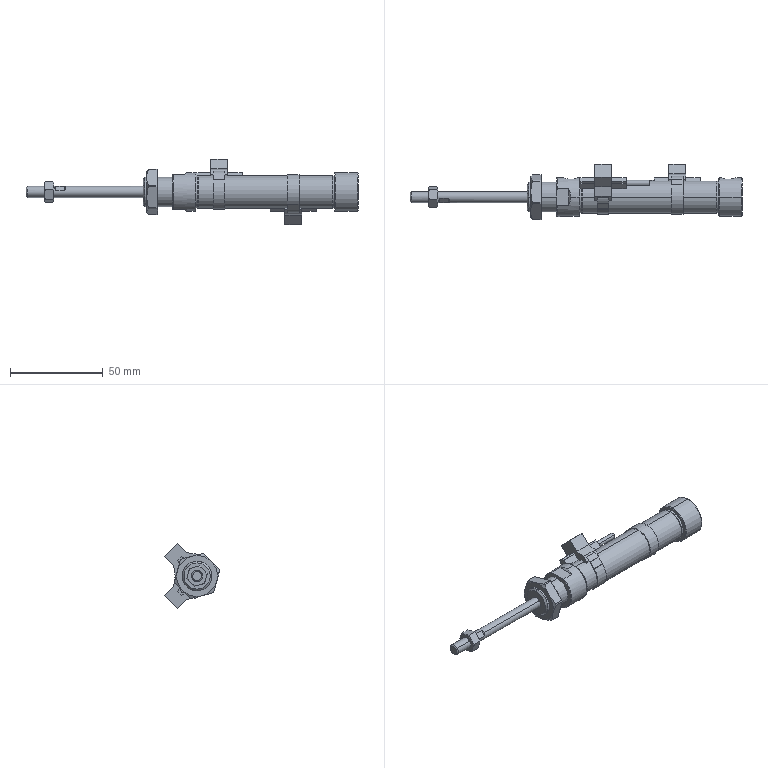Part | SolidWorks | 6 solids | 223 faces | box 179.229 x 29.769 x 35.214 mm | volume 28072 mm3 | plane 113 | cylinder 68 | cone 34 | torus 8 | commonest cylinder face diameters 17.4 x10 12.4 x8 18.4 x6 25 x6 1 x4 3 x4